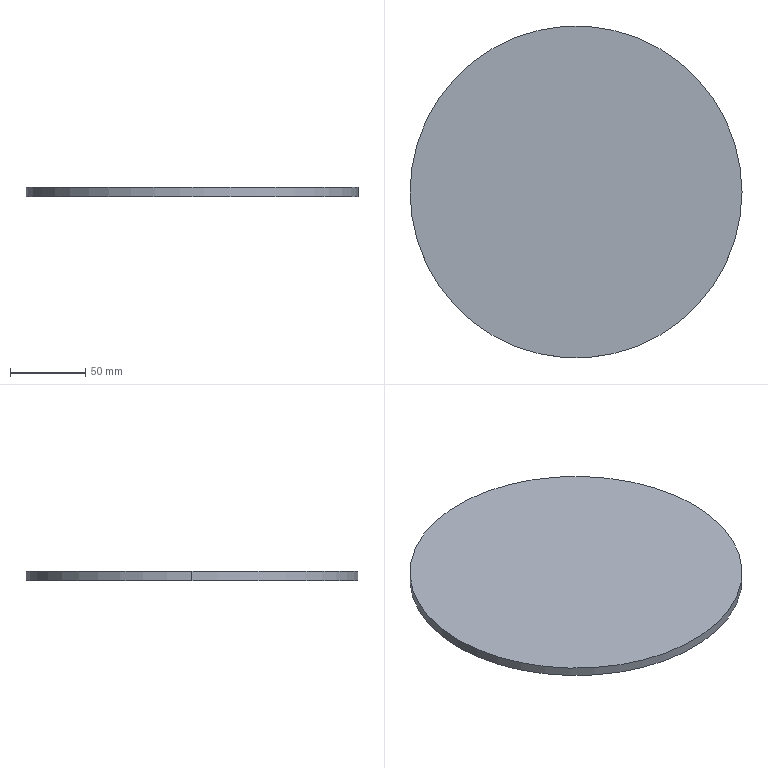Part | SolidWorks | features Extrusion 1 | 1 solid | 4 faces | box 220 x 220 x 6 mm | volume 228080 mm3 | cylinder 2 | plane 2 | commonest cylinder face diameters 220 x2
STEP:
#1=CARTESIAN_POINT('',(110.,0.,6.));
#2=VERTEX_POINT('',#1);
#3=CARTESIAN_POINT('',(-110.,0.,6.));
#4=VERTEX_POINT('',#3);
#5=CARTESIAN_POINT('',(0.,0.,6.));
#6=DIRECTION('',(0.,0.,1.));
#7=DIRECTION('',(1.,0.,0.));
#8=AXIS2_PLACEMENT_3D('',#5,#6,#7);
#9=CIRCLE('',#8,110.);
#10=EDGE_CURVE('',#2,#4,#9,.T.);
#11=ORIENTED_EDGE('',*,*,#10,.F.);
#12=CARTESIAN_POINT('',(110.,0.,0.));
#13=VERTEX_POINT('',#12);
#14=CARTESIAN_POINT('',(110.,0.,6.));
#15=DIRECTION('',(0.,0.,-1.));
#16=VECTOR('',#15,1000.);
#17=LINE('',#14,#16);
#18=EDGE_CURVE('',#2,#13,#17,.T.);
#19=ORIENTED_EDGE('',*,*,#18,.T.);
#20=CARTESIAN_POINT('',(-110.,0.,0.));
#21=VERTEX_POINT('',#20);
#22=CARTESIAN_POINT('',(0.,0.,0.));
#23=DIRECTION('',(0.,0.,1.));
#24=DIRECTION('',(1.,0.,0.));
#25=AXIS2_PLACEMENT_3D('',#22,#23,#24);
#26=CIRCLE('',#25,110.);
#27=EDGE_CURVE('',#13,#21,#26,.T.);
#28=ORIENTED_EDGE('',*,*,#27,.T.);
#29=CARTESIAN_POINT('',(-110.,0.,6.));
#30=DIRECTION('',(0.,0.,-1.));
#31=VECTOR('',#30,1000.);
#32=LINE('',#29,#31);
#33=EDGE_CURVE('',#4,#21,#32,.T.);
#34=ORIENTED_EDGE('',*,*,#33,.F.);
#35=EDGE_LOOP('',(#11,#19,#28,#34));
#36=FACE_OUTER_BOUND('',#35,.T.);
#37=CARTESIAN_POINT('',(0.,0.,6.));
#38=DIRECTION('',(0.,0.,-1.));
#39=DIRECTION('',(-1.,0.,0.));
#40=AXIS2_PLACEMENT_3D('',#37,#38,#39);
#41=CYLINDRICAL_SURFACE('',#40,110.);
#42=ADVANCED_FACE('',(#36),#41,.T.);
#43=ORIENTED_EDGE('',*,*,#18,.F.);
#44=CARTESIAN_POINT('',(0.,0.,6.));
#45=DIRECTION('',(0.,0.,1.));
#46=DIRECTION('',(1.,0.,0.));
#47=AXIS2_PLACEMENT_3D('',#44,#45,#46);
#48=CIRCLE('',#47,110.);
#49=EDGE_CURVE('',#4,#2,#48,.T.);
#50=ORIENTED_EDGE('',*,*,#49,.F.);
#51=ORIENTED_EDGE('',*,*,#33,.T.);
#52=CARTESIAN_POINT('',(0.,0.,0.));
#53=DIRECTION('',(0.,0.,1.));
#54=DIRECTION('',(1.,0.,0.));
#55=AXIS2_PLACEMENT_3D('',#52,#53,#54);
#56=CIRCLE('',#55,110.);
#57=EDGE_CURVE('',#21,#13,#56,.T.);
#58=ORIENTED_EDGE('',*,*,#57,.T.);
#59=EDGE_LOOP('',(#43,#50,#51,#58));
#60=FACE_OUTER_BOUND('',#59,.T.);
#61=CARTESIAN_POINT('',(0.,0.,6.));
#62=DIRECTION('',(0.,0.,-1.));
#63=DIRECTION('',(-1.,0.,0.));
#64=AXIS2_PLACEMENT_3D('',#61,#62,#63);
#65=CYLINDRICAL_SURFACE('',#64,110.);
#66=ADVANCED_FACE('',(#60),#65,.T.);
#67=ORIENTED_EDGE('',*,*,#49,.T.);
#68=ORIENTED_EDGE('',*,*,#10,.T.);
#69=EDGE_LOOP('',(#67,#68));
#70=FACE_OUTER_BOUND('',#69,.T.);
#71=CARTESIAN_POINT('',(0.,0.,6.));
#72=DIRECTION('',(0.,0.,1.));
#73=DIRECTION('',(1.,0.,0.));
#74=AXIS2_PLACEMENT_3D('',#71,#72,#73);
#75=PLANE('',#74);
#76=ADVANCED_FACE('',(#70),#75,.T.);
#77=ORIENTED_EDGE('',*,*,#57,.F.);
#78=ORIENTED_EDGE('',*,*,#27,.F.);
#79=EDGE_LOOP('',(#77,#78));
#80=FACE_OUTER_BOUND('',#79,.T.);
#81=CARTESIAN_POINT('',(0.,0.,0.));
#82=DIRECTION('',(0.,0.,1.));
#83=DIRECTION('',(1.,0.,0.));
#84=AXIS2_PLACEMENT_3D('',#81,#82,#83);
#85=PLANE('',#84);
#86=ADVANCED_FACE('',(#80),#85,.F.);
#87=CLOSED_SHELL('',(#42,#66,#76,#86));
#88=MANIFOLD_SOLID_BREP('',#87);
#89=CARTESIAN_POINT('',(0.,0.,0.));
#90=DIRECTION('',(0.,0.,1.));
#91=DIRECTION('',(1.,0.,0.));
#92=AXIS2_PLACEMENT_3D('',#89,#90,#91);
#93=(LENGTH_UNIT()NAMED_UNIT(*)SI_UNIT(.MILLI.,.METRE.));
#94=UNCERTAINTY_MEASURE_WITH_UNIT(LENGTH_MEASURE(0.00001),#93,'','');
#95=(NAMED_UNIT(*)PLANE_ANGLE_UNIT()SI_UNIT($,.RADIAN.));
#96=(NAMED_UNIT(*)SI_UNIT($,.STERADIAN.)SOLID_ANGLE_UNIT());
#97=(GEOMETRIC_REPRESENTATION_CONTEXT(3)GLOBAL_UNCERTAINTY_ASSIGNED_CONTEXT((#94))GLOBAL_UNIT_ASSIGNED_CONTEXT((#93,#95,#96))REPRESENTATION_CONTEXT('',''));
#98=ADVANCED_BREP_SHAPE_REPRESENTATION('',(#88,#92),#97);